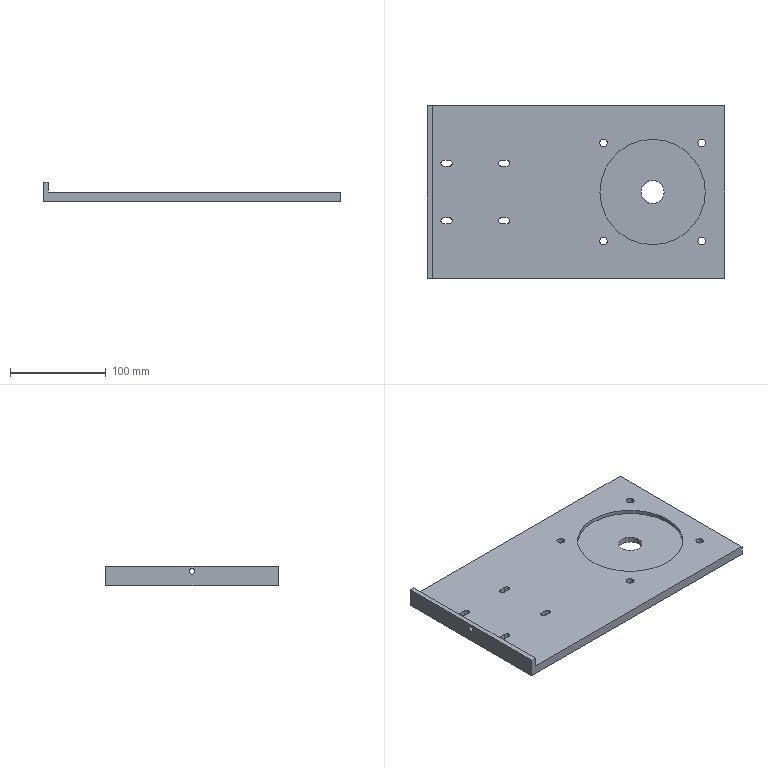Part | STEP file | Motor mounting plate | 1 solid | 43 faces | box 310 x 180 x 20 mm | volume 521549 mm3 | cylinder 26 | plane 17 | commonest cylinder face diameters 6 x14 8 x8 24 x2 110 x2
STEP:
#1=CARTESIAN_POINT('',(-36.,-56.875,10.));
#2=VERTEX_POINT('',#1);
#3=CARTESIAN_POINT('',(-33.,-53.875,10.));
#4=VERTEX_POINT('',#3);
#5=CARTESIAN_POINT('',(-33.,-56.875,10.));
#6=DIRECTION('',(0.,0.,-1.));
#7=DIRECTION('',(-1.,0.,0.));
#8=AXIS2_PLACEMENT_3D('',#5,#6,#7);
#9=CIRCLE('',#8,3.);
#10=EDGE_CURVE('',#2,#4,#9,.T.);
#11=ORIENTED_EDGE('',*,*,#10,.F.);
#12=CARTESIAN_POINT('',(-36.,-56.875,0.));
#13=VERTEX_POINT('',#12);
#14=CARTESIAN_POINT('',(-36.,-56.875,10.));
#15=DIRECTION('',(0.,0.,-1.));
#16=VECTOR('',#15,1000.);
#17=LINE('',#14,#16);
#18=EDGE_CURVE('',#2,#13,#17,.T.);
#19=ORIENTED_EDGE('',*,*,#18,.T.);
#20=CARTESIAN_POINT('',(-33.,-53.875,0.));
#21=VERTEX_POINT('',#20);
#22=CARTESIAN_POINT('',(-33.,-56.875,0.));
#23=DIRECTION('',(0.,0.,-1.));
#24=DIRECTION('',(-1.,0.,0.));
#25=AXIS2_PLACEMENT_3D('',#22,#23,#24);
#26=CIRCLE('',#25,3.);
#27=EDGE_CURVE('',#13,#21,#26,.T.);
#28=ORIENTED_EDGE('',*,*,#27,.T.);
#29=CARTESIAN_POINT('',(-33.,-53.875,10.));
#30=DIRECTION('',(0.,0.,-1.));
#31=VECTOR('',#30,1000.);
#32=LINE('',#29,#31);
#33=EDGE_CURVE('',#4,#21,#32,.T.);
#34=ORIENTED_EDGE('',*,*,#33,.F.);
#35=EDGE_LOOP('',(#11,#19,#28,#34));
#36=FACE_OUTER_BOUND('',#35,.T.);
#37=CARTESIAN_POINT('',(-33.,-56.875,10.));
#38=DIRECTION('',(0.,0.,-1.));
#39=DIRECTION('',(-1.,0.,0.));
#40=AXIS2_PLACEMENT_3D('',#37,#38,#39);
#41=CYLINDRICAL_SURFACE('',#40,3.);
#42=ADVANCED_FACE('',(#36),#41,.F.);
#43=CARTESIAN_POINT('',(-36.,3.125,10.));
#44=VERTEX_POINT('',#43);
#45=CARTESIAN_POINT('',(-33.,6.125,10.));
#46=VERTEX_POINT('',#45);
#47=CARTESIAN_POINT('',(-33.,3.125,10.));
#48=DIRECTION('',(0.,0.,-1.));
#49=DIRECTION('',(-1.,0.,0.));
#50=AXIS2_PLACEMENT_3D('',#47,#48,#49);
#51=CIRCLE('',#50,3.);
#52=EDGE_CURVE('',#44,#46,#51,.T.);
#53=ORIENTED_EDGE('',*,*,#52,.F.);
#54=CARTESIAN_POINT('',(-36.,3.125,0.));
#55=VERTEX_POINT('',#54);
#56=CARTESIAN_POINT('',(-36.,3.125,10.));
#57=DIRECTION('',(0.,0.,-1.));
#58=VECTOR('',#57,1000.);
#59=LINE('',#56,#58);
#60=EDGE_CURVE('',#44,#55,#59,.T.);
#61=ORIENTED_EDGE('',*,*,#60,.T.);
#62=CARTESIAN_POINT('',(-33.,6.125,0.));
#63=VERTEX_POINT('',#62);
#64=CARTESIAN_POINT('',(-33.,3.125,0.));
#65=DIRECTION('',(0.,0.,-1.));
#66=DIRECTION('',(-1.,0.,0.));
#67=AXIS2_PLACEMENT_3D('',#64,#65,#66);
#68=CIRCLE('',#67,3.);
#69=EDGE_CURVE('',#55,#63,#68,.T.);
#70=ORIENTED_EDGE('',*,*,#69,.T.);
#71=CARTESIAN_POINT('',(-33.,6.125,10.));
#72=DIRECTION('',(0.,0.,-1.));
#73=VECTOR('',#72,1000.);
#74=LINE('',#71,#73);
#75=EDGE_CURVE('',#46,#63,#74,.T.);
#76=ORIENTED_EDGE('',*,*,#75,.F.);
#77=EDGE_LOOP('',(#53,#61,#70,#76));
#78=FACE_OUTER_BOUND('',#77,.T.);
#79=CARTESIAN_POINT('',(-33.,3.125,10.));
#80=DIRECTION('',(0.,0.,-1.));
#81=DIRECTION('',(-1.,0.,0.));
#82=AXIS2_PLACEMENT_3D('',#79,#80,#81);
#83=CYLINDRICAL_SURFACE('',#82,3.);
#84=ADVANCED_FACE('',(#78),#83,.F.);
#85=CARTESIAN_POINT('',(240.265,-78.14,10.));
#86=VERTEX_POINT('',#85);
#87=CARTESIAN_POINT('',(232.265,-78.14,10.));
#88=VERTEX_POINT('',#87);
#89=CARTESIAN_POINT('',(236.265,-78.14,10.));
#90=DIRECTION('',(0.,0.,-1.));
#91=DIRECTION('',(-1.,0.,0.));
#92=AXIS2_PLACEMENT_3D('',#89,#90,#91);
#93=CIRCLE('',#92,4.);
#94=EDGE_CURVE('',#86,#88,#93,.T.);
#95=ORIENTED_EDGE('',*,*,#94,.F.);
#96=CARTESIAN_POINT('',(240.265,-78.14,0.));
#97=VERTEX_POINT('',#96);
#98=CARTESIAN_POINT('',(240.265,-78.14,10.));
#99=DIRECTION('',(0.,0.,-1.));
#100=VECTOR('',#99,1000.);
#101=LINE('',#98,#100);
#102=EDGE_CURVE('',#86,#97,#101,.T.);
#103=ORIENTED_EDGE('',*,*,#102,.T.);
#104=CARTESIAN_POINT('',(232.265,-78.14,0.));
#105=VERTEX_POINT('',#104);
#106=CARTESIAN_POINT('',(236.265,-78.14,0.));
#107=DIRECTION('',(0.,0.,-1.));
#108=DIRECTION('',(-1.,0.,0.));
#109=AXIS2_PLACEMENT_3D('',#106,#107,#108);
#110=CIRCLE('',#109,4.);
#111=EDGE_CURVE('',#97,#105,#110,.T.);
#112=ORIENTED_EDGE('',*,*,#111,.T.);
#113=CARTESIAN_POINT('',(232.265,-78.14,10.));
#114=DIRECTION('',(0.,0.,-1.));
#115=VECTOR('',#114,1000.);
#116=LINE('',#113,#115);
#117=EDGE_CURVE('',#88,#105,#116,.T.);
#118=ORIENTED_EDGE('',*,*,#117,.F.);
#119=EDGE_LOOP('',(#95,#103,#112,#118));
#120=FACE_OUTER_BOUND('',#119,.T.);
#121=CARTESIAN_POINT('',(236.265,-78.14,10.));
#122=DIRECTION('',(0.,0.,-1.));
#123=DIRECTION('',(-1.,0.,0.));
#124=AXIS2_PLACEMENT_3D('',#121,#122,#123);
#125=CYLINDRICAL_SURFACE('',#124,4.);
#126=ADVANCED_FACE('',(#120),#125,.F.);
#127=CARTESIAN_POINT('',(137.735,24.39,10.));
#128=VERTEX_POINT('',#127);
#129=CARTESIAN_POINT('',(129.735,24.39,10.));
#130=VERTEX_POINT('',#129);
#131=CARTESIAN_POINT('',(133.735,24.39,10.));
#132=DIRECTION('',(0.,0.,-1.));
#133=DIRECTION('',(-1.,0.,0.));
#134=AXIS2_PLACEMENT_3D('',#131,#132,#133);
#135=CIRCLE('',#134,4.);
#136=EDGE_CURVE('',#128,#130,#135,.T.);
#137=ORIENTED_EDGE('',*,*,#136,.F.);
#138=CARTESIAN_POINT('',(137.735,24.39,0.));
#139=VERTEX_POINT('',#138);
#140=CARTESIAN_POINT('',(137.735,24.39,10.));
#141=DIRECTION('',(0.,0.,-1.));
#142=VECTOR('',#141,1000.);
#143=LINE('',#140,#142);
#144=EDGE_CURVE('',#128,#139,#143,.T.);
#145=ORIENTED_EDGE('',*,*,#144,.T.);
#146=CARTESIAN_POINT('',(129.735,24.39,0.));
#147=VERTEX_POINT('',#146);
#148=CARTESIAN_POINT('',(133.735,24.39,0.));
#149=DIRECTION('',(0.,0.,-1.));
#150=DIRECTION('',(-1.,0.,0.));
#151=AXIS2_PLACEMENT_3D('',#148,#149,#150);
#152=CIRCLE('',#151,4.);
#153=EDGE_CURVE('',#139,#147,#152,.T.);
#154=ORIENTED_EDGE('',*,*,#153,.T.);
#155=CARTESIAN_POINT('',(129.735,24.39,10.));
#156=DIRECTION('',(0.,0.,-1.));
#157=VECTOR('',#156,1000.);
#158=LINE('',#155,#157);
#159=EDGE_CURVE('',#130,#147,#158,.T.);
#160=ORIENTED_EDGE('',*,*,#159,.F.);
#161=EDGE_LOOP('',(#137,#145,#154,#160));
#162=FACE_OUTER_BOUND('',#161,.T.);
#163=CARTESIAN_POINT('',(133.735,24.39,10.));
#164=DIRECTION('',(0.,0.,-1.));
#165=DIRECTION('',(-1.,0.,0.));
#166=AXIS2_PLACEMENT_3D('',#163,#164,#165);
#167=CYLINDRICAL_SURFACE('',#166,4.);
#168=ADVANCED_FACE('',(#162),#167,.F.);
#169=CARTESIAN_POINT('',(197.,-26.875,6.));
#170=VERTEX_POINT('',#169);
#171=CARTESIAN_POINT('',(173.,-26.875,6.));
#172=VERTEX_POINT('',#171);
#173=CARTESIAN_POINT('',(185.,-26.875,6.));
#174=DIRECTION('',(0.,0.,-1.));
#175=DIRECTION('',(-1.,0.,0.));
#176=AXIS2_PLACEMENT_3D('',#173,#174,#175);
#177=CIRCLE('',#176,12.);
#178=EDGE_CURVE('',#170,#172,#177,.T.);
#179=ORIENTED_EDGE('',*,*,#178,.F.);
#180=CARTESIAN_POINT('',(197.,-26.875,0.));
#181=VERTEX_POINT('',#180);
#182=CARTESIAN_POINT('',(197.,-26.875,10.));
#183=DIRECTION('',(0.,0.,-1.));
#184=VECTOR('',#183,1000.);
#185=LINE('',#182,#184);
#186=EDGE_CURVE('',#170,#181,#185,.T.);
#187=ORIENTED_EDGE('',*,*,#186,.T.);
#188=CARTESIAN_POINT('',(173.,-26.875,0.));
#189=VERTEX_POINT('',#188);
#190=CARTESIAN_POINT('',(185.,-26.875,0.));
#191=DIRECTION('',(0.,0.,-1.));
#192=DIRECTION('',(-1.,0.,0.));
#193=AXIS2_PLACEMENT_3D('',#190,#191,#192);
#194=CIRCLE('',#193,12.);
#195=EDGE_CURVE('',#181,#189,#194,.T.);
#196=ORIENTED_EDGE('',*,*,#195,.T.);
#197=CARTESIAN_POINT('',(173.,-26.875,10.));
#198=DIRECTION('',(0.,0.,-1.));
#199=VECTOR('',#198,1000.);
#200=LINE('',#197,#199);
#201=EDGE_CURVE('',#172,#189,#200,.T.);
#202=ORIENTED_EDGE('',*,*,#201,.F.);
#203=EDGE_LOOP('',(#179,#187,#196,#202));
#204=FACE_OUTER_BOUND('',#203,.T.);
#205=CARTESIAN_POINT('',(185.,-26.875,10.));
#206=DIRECTION('',(0.,0.,-1.));
#207=DIRECTION('',(-1.,0.,0.));
#208=AXIS2_PLACEMENT_3D('',#205,#206,#207);
#209=CYLINDRICAL_SURFACE('',#208,12.);
#210=ADVANCED_FACE('',(#204),#209,.F.);
#211=CARTESIAN_POINT('',(24.,3.125,10.));
#212=VERTEX_POINT('',#211);
#213=CARTESIAN_POINT('',(27.,6.125,10.));
#214=VERTEX_POINT('',#213);
#215=CARTESIAN_POINT('',(27.,3.125,10.));
#216=DIRECTION('',(0.,0.,-1.));
#217=DIRECTION('',(-1.,0.,0.));
#218=AXIS2_PLACEMENT_3D('',#215,#216,#217);
#219=CIRCLE('',#218,3.);
#220=EDGE_CURVE('',#212,#214,#219,.T.);
#221=ORIENTED_EDGE('',*,*,#220,.F.);
#222=CARTESIAN_POINT('',(24.,3.125,0.));
#223=VERTEX_POINT('',#222);
#224=CARTESIAN_POINT('',(24.,3.125,10.));
#225=DIRECTION('',(0.,0.,-1.));
#226=VECTOR('',#225,1000.);
#227=LINE('',#224,#226);
#228=EDGE_CURVE('',#212,#223,#227,.T.);
#229=ORIENTED_EDGE('',*,*,#228,.T.);
#230=CARTESIAN_POINT('',(27.,6.125,0.));
#231=VERTEX_POINT('',#230);
#232=CARTESIAN_POINT('',(27.,3.125,0.));
#233=DIRECTION('',(0.,0.,-1.));
#234=DIRECTION('',(-1.,0.,0.));
#235=AXIS2_PLACEMENT_3D('',#232,#233,#234);
#236=CIRCLE('',#235,3.);
#237=EDGE_CURVE('',#223,#231,#236,.T.);
#238=ORIENTED_EDGE('',*,*,#237,.T.);
#239=CARTESIAN_POINT('',(27.,6.125,10.));
#240=DIRECTION('',(0.,0.,-1.));
#241=VECTOR('',#240,1000.);
#242=LINE('',#239,#241);
#243=EDGE_CURVE('',#214,#231,#242,.T.);
#244=ORIENTED_EDGE('',*,*,#243,.F.);
#245=EDGE_LOOP('',(#221,#229,#238,#244));
#246=FACE_OUTER_BOUND('',#245,.T.);
#247=CARTESIAN_POINT('',(27.,3.125,10.));
#248=DIRECTION('',(0.,0.,-1.));
#249=DIRECTION('',(-1.,0.,0.));
#250=AXIS2_PLACEMENT_3D('',#247,#248,#249);
#251=CYLINDRICAL_SURFACE('',#250,3.);
#252=ADVANCED_FACE('',(#246),#251,.F.);
#253=CARTESIAN_POINT('',(240.265,24.39,10.));
#254=VERTEX_POINT('',#253);
#255=CARTESIAN_POINT('',(232.265,24.39,10.));
#256=VERTEX_POINT('',#255);
#257=CARTESIAN_POINT('',(236.265,24.39,10.));
#258=DIRECTION('',(0.,0.,-1.));
#259=DIRECTION('',(-1.,0.,0.));
#260=AXIS2_PLACEMENT_3D('',#257,#258,#259);
#261=CIRCLE('',#260,4.);
#262=EDGE_CURVE('',#254,#256,#261,.T.);
#263=ORIENTED_EDGE('',*,*,#262,.F.);
#264=CARTESIAN_POINT('',(240.265,24.39,0.));
#265=VERTEX_POINT('',#264);
#266=CARTESIAN_POINT('',(240.265,24.39,10.));
#267=DIRECTION('',(0.,0.,-1.));
#268=VECTOR('',#267,1000.);
#269=LINE('',#266,#268);
#270=EDGE_CURVE('',#254,#265,#269,.T.);
#271=ORIENTED_EDGE('',*,*,#270,.T.);
#272=CARTESIAN_POINT('',(232.265,24.39,0.));
#273=VERTEX_POINT('',#272);
#274=CARTESIAN_POINT('',(236.265,24.39,0.));
#275=DIRECTION('',(0.,0.,-1.));
#276=DIRECTION('',(-1.,0.,0.));
#277=AXIS2_PLACEMENT_3D('',#274,#275,#276);
#278=CIRCLE('',#277,4.);
#279=EDGE_CURVE('',#265,#273,#278,.T.);
#280=ORIENTED_EDGE('',*,*,#279,.T.);
#281=CARTESIAN_POINT('',(232.265,24.39,10.));
#282=DIRECTION('',(0.,0.,-1.));
#283=VECTOR('',#282,1000.);
#284=LINE('',#281,#283);
#285=EDGE_CURVE('',#256,#273,#284,.T.);
#286=ORIENTED_EDGE('',*,*,#285,.F.);
#287=EDGE_LOOP('',(#263,#271,#280,#286));
#288=FACE_OUTER_BOUND('',#287,.T.);
#289=CARTESIAN_POINT('',(236.265,24.39,10.));
#290=DIRECTION('',(0.,0.,-1.));
#291=DIRECTION('',(-1.,0.,0.));
#292=AXIS2_PLACEMENT_3D('',#289,#290,#291);
#293=CYLINDRICAL_SURFACE('',#292,4.);
#294=ADVANCED_FACE('',(#288),#293,.F.);
#295=CARTESIAN_POINT('',(137.735,-78.14,10.));
#296=VERTEX_POINT('',#295);
#297=CARTESIAN_POINT('',(129.735,-78.14,10.));
#298=VERTEX_POINT('',#297);
#299=CARTESIAN_POINT('',(133.735,-78.14,10.));
#300=DIRECTION('',(0.,0.,-1.));
#301=DIRECTION('',(-1.,0.,0.));
#302=AXIS2_PLACEMENT_3D('',#299,#300,#301);
#303=CIRCLE('',#302,4.);
#304=EDGE_CURVE('',#296,#298,#303,.T.);
#305=ORIENTED_EDGE('',*,*,#304,.F.);
#306=CARTESIAN_POINT('',(137.735,-78.14,0.));
#307=VERTEX_POINT('',#306);
#308=CARTESIAN_POINT('',(137.735,-78.14,10.));
#309=DIRECTION('',(0.,0.,-1.));
#310=VECTOR('',#309,1000.);
#311=LINE('',#308,#310);
#312=EDGE_CURVE('',#296,#307,#311,.T.);
#313=ORIENTED_EDGE('',*,*,#312,.T.);
#314=CARTESIAN_POINT('',(129.735,-78.14,0.));
#315=VERTEX_POINT('',#314);
#316=CARTESIAN_POINT('',(133.735,-78.14,0.));
#317=DIRECTION('',(0.,0.,-1.));
#318=DIRECTION('',(-1.,0.,0.));
#319=AXIS2_PLACEMENT_3D('',#316,#317,#318);
#320=CIRCLE('',#319,4.);
#321=EDGE_CURVE('',#307,#315,#320,.T.);
#322=ORIENTED_EDGE('',*,*,#321,.T.);
#323=CARTESIAN_POINT('',(129.735,-78.14,10.));
#324=DIRECTION('',(0.,0.,-1.));
#325=VECTOR('',#324,1000.);
#326=LINE('',#323,#325);
#327=EDGE_CURVE('',#298,#315,#326,.T.);
#328=ORIENTED_EDGE('',*,*,#327,.F.);
#329=EDGE_LOOP('',(#305,#313,#322,#328));
#330=FACE_OUTER_BOUND('',#329,.T.);
#331=CARTESIAN_POINT('',(133.735,-78.14,10.));
#332=DIRECTION('',(0.,0.,-1.));
#333=DIRECTION('',(-1.,0.,0.));
#334=AXIS2_PLACEMENT_3D('',#331,#332,#333);
#335=CYLINDRICAL_SURFACE('',#334,4.);
#336=ADVANCED_FACE('',(#330),#335,.F.);
#337=CARTESIAN_POINT('',(24.,-56.875,10.));
#338=VERTEX_POINT('',#337);
#339=CARTESIAN_POINT('',(27.,-53.875,10.));
#340=VERTEX_POINT('',#339);
#341=CARTESIAN_POINT('',(27.,-56.875,10.));
#342=DIRECTION('',(0.,0.,-1.));
#343=DIRECTION('',(-1.,0.,0.));
#344=AXIS2_PLACEMENT_3D('',#341,#342,#343);
#345=CIRCLE('',#344,3.);
#346=EDGE_CURVE('',#338,#340,#345,.T.);
#347=ORIENTED_EDGE('',*,*,#346,.F.);
#348=CARTESIAN_POINT('',(24.,-56.875,0.));
#349=VERTEX_POINT('',#348);
#350=CARTESIAN_POINT('',(24.,-56.875,10.));
#351=DIRECTION('',(0.,0.,-1.));
#352=VECTOR('',#351,1000.);
#353=LINE('',#350,#352);
#354=EDGE_CURVE('',#338,#349,#353,.T.);
#355=ORIENTED_EDGE('',*,*,#354,.T.);
#356=CARTESIAN_POINT('',(27.,-53.875,0.));
#357=VERTEX_POINT('',#356);
#358=CARTESIAN_POINT('',(27.,-56.875,0.));
#359=DIRECTION('',(0.,0.,-1.));
#360=DIRECTION('',(-1.,0.,0.));
#361=AXIS2_PLACEMENT_3D('',#358,#359,#360);
#362=CIRCLE('',#361,3.);
#363=EDGE_CURVE('',#349,#357,#362,.T.);
#364=ORIENTED_EDGE('',*,*,#363,.T.);
#365=CARTESIAN_POINT('',(27.,-53.875,10.));
#366=DIRECTION('',(0.,0.,-1.));
#367=VECTOR('',#366,1000.);
#368=LINE('',#365,#367);
#369=EDGE_CURVE('',#340,#357,#368,.T.);
#370=ORIENTED_EDGE('',*,*,#369,.F.);
#371=EDGE_LOOP('',(#347,#355,#364,#370));
#372=FACE_OUTER_BOUND('',#371,.T.);
#373=CARTESIAN_POINT('',(27.,-56.875,10.));
#374=DIRECTION('',(0.,0.,-1.));
#375=DIRECTION('',(-1.,0.,0.));
#376=AXIS2_PLACEMENT_3D('',#373,#374,#375);
#377=CYLINDRICAL_SURFACE('',#376,3.);
#378=ADVANCED_FACE('',(#372),#377,.F.);
#379=CARTESIAN_POINT('',(-45.,-26.875,12.));
#380=VERTEX_POINT('',#379);
#381=CARTESIAN_POINT('',(-45.,-26.875,18.));
#382=VERTEX_POINT('',#381);
#383=CARTESIAN_POINT('',(-45.,-26.875,15.));
#384=DIRECTION('',(-1.,0.,0.));
#385=DIRECTION('',(0.,0.,1.));
#386=AXIS2_PLACEMENT_3D('',#383,#384,#385);
#387=CIRCLE('',#386,3.);
#388=EDGE_CURVE('',#380,#382,#387,.T.);
#389=ORIENTED_EDGE('',*,*,#388,.F.);
#390=CARTESIAN_POINT('',(-50.,-26.875,12.));
#391=VERTEX_POINT('',#390);
#392=CARTESIAN_POINT('',(-45.,-26.875,12.));
#393=DIRECTION('',(-1.,0.,0.));
#394=VECTOR('',#393,1000.);
#395=LINE('',#392,#394);
#396=EDGE_CURVE('',#380,#391,#395,.T.);
#397=ORIENTED_EDGE('',*,*,#396,.T.);
#398=CARTESIAN_POINT('',(-50.,-26.875,18.));
#399=VERTEX_POINT('',#398);
#400=CARTESIAN_POINT('',(-50.,-26.875,15.));
#401=DIRECTION('',(-1.,0.,0.));
#402=DIRECTION('',(0.,0.,1.));
#403=AXIS2_PLACEMENT_3D('',#400,#401,#402);
#404=CIRCLE('',#403,3.);
#405=EDGE_CURVE('',#391,#399,#404,.T.);
#406=ORIENTED_EDGE('',*,*,#405,.T.);
#407=CARTESIAN_POINT('',(-45.,-26.875,18.));
#408=DIRECTION('',(-1.,0.,0.));
#409=VECTOR('',#408,1000.);
#410=LINE('',#407,#409);
#411=EDGE_CURVE('',#382,#399,#410,.T.);
#412=ORIENTED_EDGE('',*,*,#411,.F.);
#413=EDGE_LOOP('',(#389,#397,#406,#412));
#414=FACE_OUTER_BOUND('',#413,.T.);
#415=CARTESIAN_POINT('',(-45.,-26.875,15.));
#416=DIRECTION('',(-1.,0.,0.));
#417=DIRECTION('',(0.,0.,1.));
#418=AXIS2_PLACEMENT_3D('',#415,#416,#417);
#419=CYLINDRICAL_SURFACE('',#418,3.);
#420=ADVANCED_FACE('',(#414),#419,.F.);
#421=CARTESIAN_POINT('',(130.,-26.875,6.));
#422=VERTEX_POINT('',#421);
#423=CARTESIAN_POINT('',(240.,-26.875,6.));
#424=VERTEX_POINT('',#423);
#425=CARTESIAN_POINT('',(185.,-26.875,6.));
#426=DIRECTION('',(0.,0.,1.));
#427=DIRECTION('',(1.,0.,0.));
#428=AXIS2_PLACEMENT_3D('',#425,#426,#427);
#429=CIRCLE('',#428,55.);
#430=EDGE_CURVE('',#422,#424,#429,.T.);
#431=ORIENTED_EDGE('',*,*,#430,.F.);
#432=CARTESIAN_POINT('',(130.,-26.875,10.));
#433=VERTEX_POINT('',#432);
#434=CARTESIAN_POINT('',(130.,-26.875,6.));
#435=DIRECTION('',(0.,0.,1.));
#436=VECTOR('',#435,1000.);
#437=LINE('',#434,#436);
#438=EDGE_CURVE('',#422,#433,#437,.T.);
#439=ORIENTED_EDGE('',*,*,#438,.T.);
#440=CARTESIAN_POINT('',(240.,-26.875,10.));
#441=VERTEX_POINT('',#440);
#442=CARTESIAN_POINT('',(185.,-26.875,10.));
#443=DIRECTION('',(0.,0.,-1.));
#444=DIRECTION('',(1.,0.,0.));
#445=AXIS2_PLACEMENT_3D('',#442,#443,#444);
#446=CIRCLE('',#445,55.);
#447=EDGE_CURVE('',#441,#433,#446,.T.);
#448=ORIENTED_EDGE('',*,*,#447,.F.);
#449=CARTESIAN_POINT('',(240.,-26.875,6.));
#450=DIRECTION('',(0.,0.,1.));
#451=VECTOR('',#450,1000.);
#452=LINE('',#449,#451);
#453=EDGE_CURVE('',#424,#441,#452,.T.);
#454=ORIENTED_EDGE('',*,*,#453,.F.);
#455=EDGE_LOOP('',(#431,#439,#448,#454));
#456=FACE_OUTER_BOUND('',#455,.T.);
#457=CARTESIAN_POINT('',(185.,-26.875,6.));
#458=DIRECTION('',(0.,0.,1.));
#459=DIRECTION('',(1.,0.,0.));
#460=AXIS2_PLACEMENT_3D('',#457,#458,#459);
#461=CYLINDRICAL_SURFACE('',#460,55.);
#462=ADVANCED_FACE('',(#456),#461,.F.);
#463=CARTESIAN_POINT('',(-27.,-53.875,0.));
#464=VERTEX_POINT('',#463);
#465=CARTESIAN_POINT('',(-50.,-53.875,0.));
#466=DIRECTION('',(1.,0.,0.));
#467=VECTOR('',#466,1000.);
#468=LINE('',#465,#467);
#469=EDGE_CURVE('',#21,#464,#468,.T.);
#470=ORIENTED_EDGE('',*,*,#469,.F.);
#471=ORIENTED_EDGE('',*,*,#27,.F.);
#472=CARTESIAN_POINT('',(-33.,-59.875,0.));
#473=VERTEX_POINT('',#472);
#474=CARTESIAN_POINT('',(-33.,-56.875,0.));
#475=DIRECTION('',(0.,0.,-1.));
#476=DIRECTION('',(-1.,0.,0.));
#477=AXIS2_PLACEMENT_3D('',#474,#475,#476);
#478=CIRCLE('',#477,3.);
#479=EDGE_CURVE('',#473,#13,#478,.T.);
#480=ORIENTED_EDGE('',*,*,#479,.F.);
#481=CARTESIAN_POINT('',(-27.,-59.875,0.));
#482=VERTEX_POINT('',#481);
#483=CARTESIAN_POINT('',(-50.,-59.875,0.));
#484=DIRECTION('',(-1.,0.,0.));
#485=VECTOR('',#484,1000.);
#486=LINE('',#483,#485);
#487=EDGE_CURVE('',#482,#473,#486,.T.);
#488=ORIENTED_EDGE('',*,*,#487,.F.);
#489=CARTESIAN_POINT('',(-27.,-56.875,0.));
#490=DIRECTION('',(0.,0.,-1.));
#491=DIRECTION('',(-1.,0.,0.));
#492=AXIS2_PLACEMENT_3D('',#489,#490,#491);
#493=CIRCLE('',#492,3.);
#494=EDGE_CURVE('',#464,#482,#493,.T.);
#495=ORIENTED_EDGE('',*,*,#494,.F.);
#496=EDGE_LOOP('',(#470,#471,#480,#488,#495));
#497=FACE_BOUND('',#496,.T.);
#498=CARTESIAN_POINT('',(-27.,6.125,0.));
#499=VERTEX_POINT('',#498);
#500=CARTESIAN_POINT('',(-50.,6.125,0.));
#501=DIRECTION('',(1.,0.,0.));
#502=VECTOR('',#501,1000.);
#503=LINE('',#500,#502);
#504=EDGE_CURVE('',#63,#499,#503,.T.);
#505=ORIENTED_EDGE('',*,*,#504,.F.);
#506=ORIENTED_EDGE('',*,*,#69,.F.);
#507=CARTESIAN_POINT('',(-33.,0.1251,0.));
#508=VERTEX_POINT('',#507);
#509=CARTESIAN_POINT('',(-33.,3.125,0.));
#510=DIRECTION('',(0.,0.,-1.));
#511=DIRECTION('',(-1.,0.,0.));
#512=AXIS2_PLACEMENT_3D('',#509,#510,#511);
#513=CIRCLE('',#512,3.);
#514=EDGE_CURVE('',#508,#55,#513,.T.);
#515=ORIENTED_EDGE('',*,*,#514,.F.);
#516=CARTESIAN_POINT('',(-27.,0.1251,0.));
#517=VERTEX_POINT('',#516);
#518=CARTESIAN_POINT('',(-50.,0.1251,0.));
#519=DIRECTION('',(-1.,0.,0.));
#520=VECTOR('',#519,1000.);
#521=LINE('',#518,#520);
#522=EDGE_CURVE('',#517,#508,#521,.T.);
#523=ORIENTED_EDGE('',*,*,#522,.F.);
#524=CARTESIAN_POINT('',(-27.,3.125,0.));
#525=DIRECTION('',(0.,0.,-1.));
#526=DIRECTION('',(-1.,0.,0.));
#527=AXIS2_PLACEMENT_3D('',#524,#525,#526);
#528=CIRCLE('',#527,3.);
#529=EDGE_CURVE('',#499,#517,#528,.T.);
#530=ORIENTED_EDGE('',*,*,#529,.F.);
#531=EDGE_LOOP('',(#505,#506,#515,#523,#530));
#532=FACE_BOUND('',#531,.T.);
#533=CARTESIAN_POINT('',(236.265,-78.14,0.));
#534=DIRECTION('',(0.,0.,-1.));
#535=DIRECTION('',(-1.,0.,0.));
#536=AXIS2_PLACEMENT_3D('',#533,#534,#535);
#537=CIRCLE('',#536,4.);
#538=EDGE_CURVE('',#105,#97,#537,.T.);
#539=ORIENTED_EDGE('',*,*,#538,.F.);
#540=ORIENTED_EDGE('',*,*,#111,.F.);
#541=EDGE_LOOP('',(#539,#540));
#542=FACE_BOUND('',#541,.T.);
#543=CARTESIAN_POINT('',(133.735,24.39,0.));
#544=DIRECTION('',(0.,0.,-1.));
#545=DIRECTION('',(-1.,0.,0.));
#546=AXIS2_PLACEMENT_3D('',#543,#544,#545);
#547=CIRCLE('',#546,4.);
#548=EDGE_CURVE('',#147,#139,#547,.T.);
#549=ORIENTED_EDGE('',*,*,#548,.F.);
#550=ORIENTED_EDGE('',*,*,#153,.F.);
#551=EDGE_LOOP('',(#549,#550));
#552=FACE_BOUND('',#551,.T.);
#553=CARTESIAN_POINT('',(185.,-26.875,0.));
#554=DIRECTION('',(0.,0.,-1.));
#555=DIRECTION('',(-1.,0.,0.));
#556=AXIS2_PLACEMENT_3D('',#553,#554,#555);
#557=CIRCLE('',#556,12.);
#558=EDGE_CURVE('',#189,#181,#557,.T.);
#559=ORIENTED_EDGE('',*,*,#558,.F.);
#560=ORIENTED_EDGE('',*,*,#195,.F.);
#561=EDGE_LOOP('',(#559,#560));
#562=FACE_BOUND('',#561,.T.);
#563=CARTESIAN_POINT('',(260.,63.125,0.));
#564=VERTEX_POINT('',#563);
#565=CARTESIAN_POINT('',(-50.,63.125,0.));
#566=VERTEX_POINT('',#565);
#567=CARTESIAN_POINT('',(-50.,63.125,0.));
#568=DIRECTION('',(-1.,0.,0.));
#569=VECTOR('',#568,1000.);
#570=LINE('',#567,#569);
#571=EDGE_CURVE('',#564,#566,#570,.T.);
#572=ORIENTED_EDGE('',*,*,#571,.F.);
#573=CARTESIAN_POINT('',(260.,-116.875,0.));
#574=VERTEX_POINT('',#573);
#575=CARTESIAN_POINT('',(260.,-116.875,0.));
#576=DIRECTION('',(0.,1.,0.));
#577=VECTOR('',#576,1000.);
#578=LINE('',#575,#577);
#579=EDGE_CURVE('',#574,#564,#578,.T.);
#580=ORIENTED_EDGE('',*,*,#579,.F.);
#581=CARTESIAN_POINT('',(-50.,-116.875,0.));
#582=VERTEX_POINT('',#581);
#583=CARTESIAN_POINT('',(-50.,-116.875,0.));
#584=DIRECTION('',(1.,0.,0.));
#585=VECTOR('',#584,1000.);
#586=LINE('',#583,#585);
#587=EDGE_CURVE('',#582,#574,#586,.T.);
#588=ORIENTED_EDGE('',*,*,#587,.F.);
#589=CARTESIAN_POINT('',(-50.,-116.875,0.));
#590=DIRECTION('',(0.,-1.,0.));
#591=VECTOR('',#590,1000.);
#592=LINE('',#589,#591);
#593=EDGE_CURVE('',#566,#582,#592,.T.);
#594=ORIENTED_EDGE('',*,*,#593,.F.);
#595=EDGE_LOOP('',(#572,#580,#588,#594));
#596=FACE_OUTER_BOUND('',#595,.T.);
#597=CARTESIAN_POINT('',(33.,6.125,0.));
#598=VERTEX_POINT('',#597);
#599=CARTESIAN_POINT('',(-50.,6.125,0.));
#600=DIRECTION('',(1.,0.,0.));
#601=VECTOR('',#600,1000.);
#602=LINE('',#599,#601);
#603=EDGE_CURVE('',#231,#598,#602,.T.);
#604=ORIENTED_EDGE('',*,*,#603,.F.);
#605=ORIENTED_EDGE('',*,*,#237,.F.);
#606=CARTESIAN_POINT('',(27.,0.1251,0.));
#607=VERTEX_POINT('',#606);
#608=CARTESIAN_POINT('',(27.,3.125,0.));
#609=DIRECTION('',(0.,0.,-1.));
#610=DIRECTION('',(-1.,0.,0.));
#611=AXIS2_PLACEMENT_3D('',#608,#609,#610);
#612=CIRCLE('',#611,3.);
#613=EDGE_CURVE('',#607,#223,#612,.T.);
#614=ORIENTED_EDGE('',*,*,#613,.F.);
#615=CARTESIAN_POINT('',(33.,0.1251,0.));
#616=VERTEX_POINT('',#615);
#617=CARTESIAN_POINT('',(-50.,0.1251,0.));
#618=DIRECTION('',(-1.,0.,0.));
#619=VECTOR('',#618,1000.);
#620=LINE('',#617,#619);
#621=EDGE_CURVE('',#616,#607,#620,.T.);
#622=ORIENTED_EDGE('',*,*,#621,.F.);
#623=CARTESIAN_POINT('',(33.,3.125,0.));
#624=DIRECTION('',(0.,0.,-1.));
#625=DIRECTION('',(-1.,0.,0.));
#626=AXIS2_PLACEMENT_3D('',#623,#624,#625);
#627=CIRCLE('',#626,3.);
#628=EDGE_CURVE('',#598,#616,#627,.T.);
#629=ORIENTED_EDGE('',*,*,#628,.F.);
#630=EDGE_LOOP('',(#604,#605,#614,#622,#629));
#631=FACE_BOUND('',#630,.T.);
#632=CARTESIAN_POINT('',(236.265,24.39,0.));
#633=DIRECTION('',(0.,0.,-1.));
#634=DIRECTION('',(-1.,0.,0.));
#635=AXIS2_PLACEMENT_3D('',#632,#633,#634);
#636=CIRCLE('',#635,4.);
#637=EDGE_CURVE('',#273,#265,#636,.T.);
#638=ORIENTED_EDGE('',*,*,#637,.F.);
#639=ORIENTED_EDGE('',*,*,#279,.F.);
#640=EDGE_LOOP('',(#638,#639));
#641=FACE_BOUND('',#640,.T.);
#642=CARTESIAN_POINT('',(133.735,-78.14,0.));
#643=DIRECTION('',(0.,0.,-1.));
#644=DIRECTION('',(-1.,0.,0.));
#645=AXIS2_PLACEMENT_3D('',#642,#643,#644);
#646=CIRCLE('',#645,4.);
#647=EDGE_CURVE('',#315,#307,#646,.T.);
#648=ORIENTED_EDGE('',*,*,#647,.F.);
#649=ORIENTED_EDGE('',*,*,#321,.F.);
#650=EDGE_LOOP('',(#648,#649));
#651=FACE_BOUND('',#650,.T.);
#652=CARTESIAN_POINT('',(33.,-53.875,0.));
#653=VERTEX_POINT('',#652);
#654=CARTESIAN_POINT('',(-50.,-53.875,0.));
#655=DIRECTION('',(1.,0.,0.));
#656=VECTOR('',#655,1000.);
#657=LINE('',#654,#656);
#658=EDGE_CURVE('',#357,#653,#657,.T.);
#659=ORIENTED_EDGE('',*,*,#658,.F.);
#660=ORIENTED_EDGE('',*,*,#363,.F.);
#661=CARTESIAN_POINT('',(27.,-59.875,0.));
#662=VERTEX_POINT('',#661);
#663=CARTESIAN_POINT('',(27.,-56.875,0.));
#664=DIRECTION('',(0.,0.,-1.));
#665=DIRECTION('',(-1.,0.,0.));
#666=AXIS2_PLACEMENT_3D('',#663,#664,#665);
#667=CIRCLE('',#666,3.);
#668=EDGE_CURVE('',#662,#349,#667,.T.);
#669=ORIENTED_EDGE('',*,*,#668,.F.);
#670=CARTESIAN_POINT('',(33.,-59.875,0.));
#671=VERTEX_POINT('',#670);
#672=CARTESIAN_POINT('',(-50.,-59.875,0.));
#673=DIRECTION('',(-1.,0.,0.));
#674=VECTOR('',#673,1000.);
#675=LINE('',#672,#674);
#676=EDGE_CURVE('',#671,#662,#675,.T.);
#677=ORIENTED_EDGE('',*,*,#676,.F.);
#678=CARTESIAN_POINT('',(33.,-56.875,0.));
#679=DIRECTION('',(0.,0.,-1.));
#680=DIRECTION('',(-1.,0.,0.));
#681=AXIS2_PLACEMENT_3D('',#678,#679,#680);
#682=CIRCLE('',#681,3.);
#683=EDGE_CURVE('',#653,#671,#682,.T.);
#684=ORIENTED_EDGE('',*,*,#683,.F.);
#685=EDGE_LOOP('',(#659,#660,#669,#677,#684));
#686=FACE_BOUND('',#685,.T.);
#687=CARTESIAN_POINT('',(-50.,-116.875,0.));
#688=DIRECTION('',(0.,0.,1.));
#689=DIRECTION('',(1.,0.,0.));
#690=AXIS2_PLACEMENT_3D('',#687,#688,#689);
#691=PLANE('',#690);
#692=ADVANCED_FACE('',(#497,#532,#542,#552,#562,#596,#631,#641,#651,#686),#691,.F.);
#693=CARTESIAN_POINT('',(-27.,-59.875,10.));
#694=VERTEX_POINT('',#693);
#695=CARTESIAN_POINT('',(-27.,-59.875,10.));
#696=DIRECTION('',(0.,0.,-1.));
#697=VECTOR('',#696,1000.);
#698=LINE('',#695,#697);
#699=EDGE_CURVE('',#694,#482,#698,.T.);
#700=ORIENTED_EDGE('',*,*,#699,.F.);
#701=CARTESIAN_POINT('',(-27.,-53.875,10.));
#702=VERTEX_POINT('',#701);
#703=CARTESIAN_POINT('',(-27.,-56.875,10.));
#704=DIRECTION('',(0.,0.,-1.));
#705=DIRECTION('',(-1.,0.,0.));
#706=AXIS2_PLACEMENT_3D('',#703,#704,#705);
#707=CIRCLE('',#706,3.);
#708=EDGE_CURVE('',#702,#694,#707,.T.);
#709=ORIENTED_EDGE('',*,*,#708,.F.);
#710=CARTESIAN_POINT('',(-27.,-53.875,10.));
#711=DIRECTION('',(0.,0.,1.));
#712=VECTOR('',#711,1000.);
#713=LINE('',#710,#712);
#714=EDGE_CURVE('',#464,#702,#713,.T.);
#715=ORIENTED_EDGE('',*,*,#714,.F.);
#716=ORIENTED_EDGE('',*,*,#494,.T.);
#717=EDGE_LOOP('',(#700,#709,#715,#716));
#718=FACE_OUTER_BOUND('',#717,.T.);
#719=CARTESIAN_POINT('',(-27.,-56.875,10.));
#720=DIRECTION('',(0.,0.,-1.));
#721=DIRECTION('',(-1.,0.,0.));
#722=AXIS2_PLACEMENT_3D('',#719,#720,#721);
#723=CYLINDRICAL_SURFACE('',#722,3.);
#724=ADVANCED_FACE('',(#718),#723,.F.);
#725=CARTESIAN_POINT('',(-27.,-53.875,10.));
#726=DIRECTION('',(-1.,0.,0.));
#727=VECTOR('',#726,1000.);
#728=LINE('',#725,#727);
#729=EDGE_CURVE('',#702,#4,#728,.T.);
#730=ORIENTED_EDGE('',*,*,#729,.T.);
#731=ORIENTED_EDGE('',*,*,#33,.T.);
#732=ORIENTED_EDGE('',*,*,#469,.T.);
#733=ORIENTED_EDGE('',*,*,#714,.T.);
#734=EDGE_LOOP('',(#730,#731,#732,#733));
#735=FACE_OUTER_BOUND('',#734,.T.);
#736=CARTESIAN_POINT('',(-27.,-53.875,10.));
#737=DIRECTION('',(0.,-1.,0.));
#738=DIRECTION('',(0.,0.,-1.));
#739=AXIS2_PLACEMENT_3D('',#736,#737,#738);
#740=PLANE('',#739);
#741=ADVANCED_FACE('',(#735),#740,.T.);
#742=ORIENTED_EDGE('',*,*,#18,.F.);
#743=CARTESIAN_POINT('',(-33.,-59.875,10.));
#744=VERTEX_POINT('',#743);
#745=CARTESIAN_POINT('',(-33.,-56.875,10.));
#746=DIRECTION('',(0.,0.,-1.));
#747=DIRECTION('',(-1.,0.,0.));
#748=AXIS2_PLACEMENT_3D('',#745,#746,#747);
#749=CIRCLE('',#748,3.);
#750=EDGE_CURVE('',#744,#2,#749,.T.);
#751=ORIENTED_EDGE('',*,*,#750,.F.);
#752=CARTESIAN_POINT('',(-33.,-59.875,10.));
#753=DIRECTION('',(0.,0.,1.));
#754=VECTOR('',#753,1000.);
#755=LINE('',#752,#754);
#756=EDGE_CURVE('',#473,#744,#755,.T.);
#757=ORIENTED_EDGE('',*,*,#756,.F.);
#758=ORIENTED_EDGE('',*,*,#479,.T.);
#759=EDGE_LOOP('',(#742,#751,#757,#758));
#760=FACE_OUTER_BOUND('',#759,.T.);
#761=CARTESIAN_POINT('',(-33.,-56.875,10.));
#762=DIRECTION('',(0.,0.,-1.));
#763=DIRECTION('',(-1.,0.,0.));
#764=AXIS2_PLACEMENT_3D('',#761,#762,#763);
#765=CYLINDRICAL_SURFACE('',#764,3.);
#766=ADVANCED_FACE('',(#760),#765,.F.);
#767=CARTESIAN_POINT('',(-27.,-59.875,10.));
#768=DIRECTION('',(1.,0.,0.));
#769=VECTOR('',#768,1000.);
#770=LINE('',#767,#769);
#771=EDGE_CURVE('',#744,#694,#770,.T.);
#772=ORIENTED_EDGE('',*,*,#771,.T.);
#773=ORIENTED_EDGE('',*,*,#699,.T.);
#774=ORIENTED_EDGE('',*,*,#487,.T.);
#775=ORIENTED_EDGE('',*,*,#756,.T.);
#776=EDGE_LOOP('',(#772,#773,#774,#775));
#777=FACE_OUTER_BOUND('',#776,.T.);
#778=CARTESIAN_POINT('',(-27.,-59.875,10.));
#779=DIRECTION('',(0.,1.,0.));
#780=DIRECTION('',(0.,0.,1.));
#781=AXIS2_PLACEMENT_3D('',#778,#779,#780);
#782=PLANE('',#781);
#783=ADVANCED_FACE('',(#777),#782,.T.);
#784=CARTESIAN_POINT('',(-27.,0.1251,10.));
#785=VERTEX_POINT('',#784);
#786=CARTESIAN_POINT('',(-27.,0.1251,10.));
#787=DIRECTION('',(0.,0.,-1.));
#788=VECTOR('',#787,1000.);
#789=LINE('',#786,#788);
#790=EDGE_CURVE('',#785,#517,#789,.T.);
#791=ORIENTED_EDGE('',*,*,#790,.F.);
#792=CARTESIAN_POINT('',(-27.,6.125,10.));
#793=VERTEX_POINT('',#792);
#794=CARTESIAN_POINT('',(-27.,3.125,10.));
#795=DIRECTION('',(0.,0.,-1.));
#796=DIRECTION('',(-1.,0.,0.));
#797=AXIS2_PLACEMENT_3D('',#794,#795,#796);
#798=CIRCLE('',#797,3.);
#799=EDGE_CURVE('',#793,#785,#798,.T.);
#800=ORIENTED_EDGE('',*,*,#799,.F.);
#801=CARTESIAN_POINT('',(-27.,6.125,10.));
#802=DIRECTION('',(0.,0.,1.));
#803=VECTOR('',#802,1000.);
#804=LINE('',#801,#803);
#805=EDGE_CURVE('',#499,#793,#804,.T.);
#806=ORIENTED_EDGE('',*,*,#805,.F.);
#807=ORIENTED_EDGE('',*,*,#529,.T.);
#808=EDGE_LOOP('',(#791,#800,#806,#807));
#809=FACE_OUTER_BOUND('',#808,.T.);
#810=CARTESIAN_POINT('',(-27.,3.125,10.));
#811=DIRECTION('',(0.,0.,-1.));
#812=DIRECTION('',(-1.,0.,0.));
#813=AXIS2_PLACEMENT_3D('',#810,#811,#812);
#814=CYLINDRICAL_SURFACE('',#813,3.);
#815=ADVANCED_FACE('',(#809),#814,.F.);
#816=CARTESIAN_POINT('',(-27.,6.125,10.));
#817=DIRECTION('',(-1.,0.,0.));
#818=VECTOR('',#817,1000.);
#819=LINE('',#816,#818);
#820=EDGE_CURVE('',#793,#46,#819,.T.);
#821=ORIENTED_EDGE('',*,*,#820,.T.);
#822=ORIENTED_EDGE('',*,*,#75,.T.);
#823=ORIENTED_EDGE('',*,*,#504,.T.);
#824=ORIENTED_EDGE('',*,*,#805,.T.);
#825=EDGE_LOOP('',(#821,#822,#823,#824));
#826=FACE_OUTER_BOUND('',#825,.T.);
#827=CARTESIAN_POINT('',(-27.,6.125,10.));
#828=DIRECTION('',(0.,-1.,0.));
#829=DIRECTION('',(0.,0.,-1.));
#830=AXIS2_PLACEMENT_3D('',#827,#828,#829);
#831=PLANE('',#830);
#832=ADVANCED_FACE('',(#826),#831,.T.);
#833=ORIENTED_EDGE('',*,*,#60,.F.);
#834=CARTESIAN_POINT('',(-33.,0.1251,10.));
#835=VERTEX_POINT('',#834);
#836=CARTESIAN_POINT('',(-33.,3.125,10.));
#837=DIRECTION('',(0.,0.,-1.));
#838=DIRECTION('',(-1.,0.,0.));
#839=AXIS2_PLACEMENT_3D('',#836,#837,#838);
#840=CIRCLE('',#839,3.);
#841=EDGE_CURVE('',#835,#44,#840,.T.);
#842=ORIENTED_EDGE('',*,*,#841,.F.);
#843=CARTESIAN_POINT('',(-33.,0.1251,10.));
#844=DIRECTION('',(0.,0.,1.));
#845=VECTOR('',#844,1000.);
#846=LINE('',#843,#845);
#847=EDGE_CURVE('',#508,#835,#846,.T.);
#848=ORIENTED_EDGE('',*,*,#847,.F.);
#849=ORIENTED_EDGE('',*,*,#514,.T.);
#850=EDGE_LOOP('',(#833,#842,#848,#849));
#851=FACE_OUTER_BOUND('',#850,.T.);
#852=CARTESIAN_POINT('',(-33.,3.125,10.));
#853=DIRECTION('',(0.,0.,-1.));
#854=DIRECTION('',(-1.,0.,0.));
#855=AXIS2_PLACEMENT_3D('',#852,#853,#854);
#856=CYLINDRICAL_SURFACE('',#855,3.);
#857=ADVANCED_FACE('',(#851),#856,.F.);
#858=CARTESIAN_POINT('',(-27.,0.1251,10.));
#859=DIRECTION('',(1.,0.,0.));
#860=VECTOR('',#859,1000.);
#861=LINE('',#858,#860);
#862=EDGE_CURVE('',#835,#785,#861,.T.);
#863=ORIENTED_EDGE('',*,*,#862,.T.);
#864=ORIENTED_EDGE('',*,*,#790,.T.);
#865=ORIENTED_EDGE('',*,*,#522,.T.);
#866=ORIENTED_EDGE('',*,*,#847,.T.);
#867=EDGE_LOOP('',(#863,#864,#865,#866));
#868=FACE_OUTER_BOUND('',#867,.T.);
#869=CARTESIAN_POINT('',(-27.,0.1251,10.));
#870=DIRECTION('',(0.,1.,0.));
#871=DIRECTION('',(0.,0.,1.));
#872=AXIS2_PLACEMENT_3D('',#869,#870,#871);
#873=PLANE('',#872);
#874=ADVANCED_FACE('',(#868),#873,.T.);
#875=ORIENTED_EDGE('',*,*,#102,.F.);
#876=CARTESIAN_POINT('',(236.265,-78.14,10.));
#877=DIRECTION('',(0.,0.,-1.));
#878=DIRECTION('',(-1.,0.,0.));
#879=AXIS2_PLACEMENT_3D('',#876,#877,#878);
#880=CIRCLE('',#879,4.);
#881=EDGE_CURVE('',#88,#86,#880,.T.);
#882=ORIENTED_EDGE('',*,*,#881,.F.);
#883=ORIENTED_EDGE('',*,*,#117,.T.);
#884=ORIENTED_EDGE('',*,*,#538,.T.);
#885=EDGE_LOOP('',(#875,#882,#883,#884));
#886=FACE_OUTER_BOUND('',#885,.T.);
#887=CARTESIAN_POINT('',(236.265,-78.14,10.));
#888=DIRECTION('',(0.,0.,-1.));
#889=DIRECTION('',(-1.,0.,0.));
#890=AXIS2_PLACEMENT_3D('',#887,#888,#889);
#891=CYLINDRICAL_SURFACE('',#890,4.);
#892=ADVANCED_FACE('',(#886),#891,.F.);
#893=ORIENTED_EDGE('',*,*,#144,.F.);
#894=CARTESIAN_POINT('',(133.735,24.39,10.));
#895=DIRECTION('',(0.,0.,-1.));
#896=DIRECTION('',(-1.,0.,0.));
#897=AXIS2_PLACEMENT_3D('',#894,#895,#896);
#898=CIRCLE('',#897,4.);
#899=EDGE_CURVE('',#130,#128,#898,.T.);
#900=ORIENTED_EDGE('',*,*,#899,.F.);
#901=ORIENTED_EDGE('',*,*,#159,.T.);
#902=ORIENTED_EDGE('',*,*,#548,.T.);
#903=EDGE_LOOP('',(#893,#900,#901,#902));
#904=FACE_OUTER_BOUND('',#903,.T.);
#905=CARTESIAN_POINT('',(133.735,24.39,10.));
#906=DIRECTION('',(0.,0.,-1.));
#907=DIRECTION('',(-1.,0.,0.));
#908=AXIS2_PLACEMENT_3D('',#905,#906,#907);
#909=CYLINDRICAL_SURFACE('',#908,4.);
#910=ADVANCED_FACE('',(#904),#909,.F.);
#911=ORIENTED_EDGE('',*,*,#186,.F.);
#912=CARTESIAN_POINT('',(185.,-26.875,6.));
#913=DIRECTION('',(0.,0.,-1.));
#914=DIRECTION('',(-1.,0.,0.));
#915=AXIS2_PLACEMENT_3D('',#912,#913,#914);
#916=CIRCLE('',#915,12.);
#917=EDGE_CURVE('',#172,#170,#916,.T.);
#918=ORIENTED_EDGE('',*,*,#917,.F.);
#919=ORIENTED_EDGE('',*,*,#201,.T.);
#920=ORIENTED_EDGE('',*,*,#558,.T.);
#921=EDGE_LOOP('',(#911,#918,#919,#920));
#922=FACE_OUTER_BOUND('',#921,.T.);
#923=CARTESIAN_POINT('',(185.,-26.875,10.));
#924=DIRECTION('',(0.,0.,-1.));
#925=DIRECTION('',(-1.,0.,0.));
#926=AXIS2_PLACEMENT_3D('',#923,#924,#925);
#927=CYLINDRICAL_SURFACE('',#926,12.);
#928=ADVANCED_FACE('',(#922),#927,.F.);
#929=CARTESIAN_POINT('',(-50.,-26.875,15.));
#930=DIRECTION('',(-1.,0.,0.));
#931=DIRECTION('',(0.,0.,1.));
#932=AXIS2_PLACEMENT_3D('',#929,#930,#931);
#933=CIRCLE('',#932,3.);
#934=EDGE_CURVE('',#399,#391,#933,.T.);
#935=ORIENTED_EDGE('',*,*,#934,.F.);
#936=ORIENTED_EDGE('',*,*,#405,.F.);
#937=EDGE_LOOP('',(#935,#936));
#938=FACE_BOUND('',#937,.T.);
#939=CARTESIAN_POINT('',(-50.,-116.875,20.));
#940=VERTEX_POINT('',#939);
#941=CARTESIAN_POINT('',(-50.,-116.875,10.));
#942=DIRECTION('',(0.,0.,-1.));
#943=VECTOR('',#942,1000.);
#944=LINE('',#941,#943);
#945=EDGE_CURVE('',#940,#582,#944,.T.);
#946=ORIENTED_EDGE('',*,*,#945,.F.);
#947=CARTESIAN_POINT('',(-50.,63.125,20.));
#948=VERTEX_POINT('',#947);
#949=CARTESIAN_POINT('',(-50.,63.125,20.));
#950=DIRECTION('',(0.,-1.,0.));
#951=VECTOR('',#950,1000.);
#952=LINE('',#949,#951);
#953=EDGE_CURVE('',#948,#940,#952,.T.);
#954=ORIENTED_EDGE('',*,*,#953,.F.);
#955=CARTESIAN_POINT('',(-50.,63.125,10.));
#956=DIRECTION('',(0.,0.,1.));
#957=VECTOR('',#956,1000.);
#958=LINE('',#955,#957);
#959=EDGE_CURVE('',#566,#948,#958,.T.);
#960=ORIENTED_EDGE('',*,*,#959,.F.);
#961=ORIENTED_EDGE('',*,*,#593,.T.);
#962=EDGE_LOOP('',(#946,#954,#960,#961));
#963=FACE_OUTER_BOUND('',#962,.T.);
#964=CARTESIAN_POINT('',(-50.,63.125,10.));
#965=DIRECTION('',(1.,0.,0.));
#966=DIRECTION('',(0.,1.,0.));
#967=AXIS2_PLACEMENT_3D('',#964,#965,#966);
#968=PLANE('',#967);
#969=ADVANCED_FACE('',(#938,#963),#968,.F.);
#970=ORIENTED_EDGE('',*,*,#959,.T.);
#971=CARTESIAN_POINT('',(-45.,63.125,20.));
#972=VERTEX_POINT('',#971);
#973=CARTESIAN_POINT('',(-50.,63.125,20.));
#974=DIRECTION('',(-1.,0.,0.));
#975=VECTOR('',#974,1000.);
#976=LINE('',#973,#975);
#977=EDGE_CURVE('',#972,#948,#976,.T.);
#978=ORIENTED_EDGE('',*,*,#977,.F.);
#979=CARTESIAN_POINT('',(-45.,63.125,10.));
#980=VERTEX_POINT('',#979);
#981=CARTESIAN_POINT('',(-45.,63.125,10.));
#982=DIRECTION('',(0.,0.,1.));
#983=VECTOR('',#982,1000.);
#984=LINE('',#981,#983);
#985=EDGE_CURVE('',#980,#972,#984,.T.);
#986=ORIENTED_EDGE('',*,*,#985,.F.);
#987=CARTESIAN_POINT('',(260.,63.125,10.));
#988=VERTEX_POINT('',#987);
#989=CARTESIAN_POINT('',(-50.,63.125,10.));
#990=DIRECTION('',(-1.,0.,0.));
#991=VECTOR('',#990,1000.);
#992=LINE('',#989,#991);
#993=EDGE_CURVE('',#988,#980,#992,.T.);
#994=ORIENTED_EDGE('',*,*,#993,.F.);
#995=CARTESIAN_POINT('',(260.,63.125,10.));
#996=DIRECTION('',(0.,0.,1.));
#997=VECTOR('',#996,1000.);
#998=LINE('',#995,#997);
#999=EDGE_CURVE('',#564,#988,#998,.T.);
#1000=ORIENTED_EDGE('',*,*,#999,.F.);
#1001=ORIENTED_EDGE('',*,*,#571,.T.);
#1002=EDGE_LOOP('',(#970,#978,#986,#994,#1000,#1001));
#1003=FACE_OUTER_BOUND('',#1002,.T.);
#1004=CARTESIAN_POINT('',(-50.,63.125,10.));
#1005=DIRECTION('',(0.,-1.,0.));
#1006=DIRECTION('',(0.,0.,-1.));
#1007=AXIS2_PLACEMENT_3D('',#1004,#1005,#1006);
#1008=PLANE('',#1007);
#1009=ADVANCED_FACE('',(#1003),#1008,.F.);
#1010=ORIENTED_EDGE('',*,*,#999,.T.);
#1011=CARTESIAN_POINT('',(260.,-116.875,10.));
#1012=VERTEX_POINT('',#1011);
#1013=CARTESIAN_POINT('',(260.,63.125,10.));
#1014=DIRECTION('',(0.,1.,0.));
#1015=VECTOR('',#1014,1000.);
#1016=LINE('',#1013,#1015);
#1017=EDGE_CURVE('',#1012,#988,#1016,.T.);
#1018=ORIENTED_EDGE('',*,*,#1017,.F.);
#1019=CARTESIAN_POINT('',(260.,-116.875,10.));
#1020=DIRECTION('',(0.,0.,1.));
#1021=VECTOR('',#1020,1000.);
#1022=LINE('',#1019,#1021);
#1023=EDGE_CURVE('',#574,#1012,#1022,.T.);
#1024=ORIENTED_EDGE('',*,*,#1023,.F.);
#1025=ORIENTED_EDGE('',*,*,#579,.T.);
#1026=EDGE_LOOP('',(#1010,#1018,#1024,#1025));
#1027=FACE_OUTER_BOUND('',#1026,.T.);
#1028=CARTESIAN_POINT('',(260.,63.125,10.));
#1029=DIRECTION('',(-1.,0.,0.));
#1030=DIRECTION('',(0.,0.,1.));
#1031=AXIS2_PLACEMENT_3D('',#1028,#1029,#1030);
#1032=PLANE('',#1031);
#1033=ADVANCED_FACE('',(#1027),#1032,.F.);
#1034=ORIENTED_EDGE('',*,*,#1023,.T.);
#1035=CARTESIAN_POINT('',(-45.,-116.875,10.));
#1036=VERTEX_POINT('',#1035);
#1037=CARTESIAN_POINT('',(-50.,-116.875,10.));
#1038=DIRECTION('',(1.,0.,0.));
#1039=VECTOR('',#1038,1000.);
#1040=LINE('',#1037,#1039);
#1041=EDGE_CURVE('',#1036,#1012,#1040,.T.);
#1042=ORIENTED_EDGE('',*,*,#1041,.F.);
#1043=CARTESIAN_POINT('',(-45.,-116.875,20.));
#1044=VERTEX_POINT('',#1043);
#1045=CARTESIAN_POINT('',(-45.,-116.875,10.));
#1046=DIRECTION('',(0.,0.,-1.));
#1047=VECTOR('',#1046,1000.);
#1048=LINE('',#1045,#1047);
#1049=EDGE_CURVE('',#1044,#1036,#1048,.T.);
#1050=ORIENTED_EDGE('',*,*,#1049,.F.);
#1051=CARTESIAN_POINT('',(-50.,-116.875,20.));
#1052=DIRECTION('',(1.,0.,0.));
#1053=VECTOR('',#1052,1000.);
#1054=LINE('',#1051,#1053);
#1055=EDGE_CURVE('',#940,#1044,#1054,.T.);
#1056=ORIENTED_EDGE('',*,*,#1055,.F.);
#1057=ORIENTED_EDGE('',*,*,#945,.T.);
#1058=ORIENTED_EDGE('',*,*,#587,.T.);
#1059=EDGE_LOOP('',(#1034,#1042,#1050,#1056,#1057,#1058));
#1060=FACE_OUTER_BOUND('',#1059,.T.);
#1061=CARTESIAN_POINT('',(-50.,-116.875,10.));
#1062=DIRECTION('',(0.,1.,0.));
#1063=DIRECTION('',(0.,0.,1.));
#1064=AXIS2_PLACEMENT_3D('',#1061,#1062,#1063);
#1065=PLANE('',#1064);
#1066=ADVANCED_FACE('',(#1060),#1065,.F.);
#1067=CARTESIAN_POINT('',(33.,0.1251,10.));
#1068=VERTEX_POINT('',#1067);
#1069=CARTESIAN_POINT('',(33.,0.1251,10.));
#1070=DIRECTION('',(0.,0.,-1.));
#1071=VECTOR('',#1070,1000.);
#1072=LINE('',#1069,#1071);
#1073=EDGE_CURVE('',#1068,#616,#1072,.T.);
#1074=ORIENTED_EDGE('',*,*,#1073,.F.);
#1075=CARTESIAN_POINT('',(33.,6.125,10.));
#1076=VERTEX_POINT('',#1075);
#1077=CARTESIAN_POINT('',(33.,3.125,10.));
#1078=DIRECTION('',(0.,0.,-1.));
#1079=DIRECTION('',(-1.,0.,0.));
#1080=AXIS2_PLACEMENT_3D('',#1077,#1078,#1079);
#1081=CIRCLE('',#1080,3.);
#1082=EDGE_CURVE('',#1076,#1068,#1081,.T.);
#1083=ORIENTED_EDGE('',*,*,#1082,.F.);
#1084=CARTESIAN_POINT('',(33.,6.125,10.));
#1085=DIRECTION('',(0.,0.,1.));
#1086=VECTOR('',#1085,1000.);
#1087=LINE('',#1084,#1086);
#1088=EDGE_CURVE('',#598,#1076,#1087,.T.);
#1089=ORIENTED_EDGE('',*,*,#1088,.F.);
#1090=ORIENTED_EDGE('',*,*,#628,.T.);
#1091=EDGE_LOOP('',(#1074,#1083,#1089,#1090));
#1092=FACE_OUTER_BOUND('',#1091,.T.);
#1093=CARTESIAN_POINT('',(33.,3.125,10.));
#1094=DIRECTION('',(0.,0.,-1.));
#1095=DIRECTION('',(-1.,0.,0.));
#1096=AXIS2_PLACEMENT_3D('',#1093,#1094,#1095);
#1097=CYLINDRICAL_SURFACE('',#1096,3.);
#1098=ADVANCED_FACE('',(#1092),#1097,.F.);
#1099=CARTESIAN_POINT('',(33.,6.125,10.));
#1100=DIRECTION('',(-1.,0.,0.));
#1101=VECTOR('',#1100,1000.);
#1102=LINE('',#1099,#1101);
#1103=EDGE_CURVE('',#1076,#214,#1102,.T.);
#1104=ORIENTED_EDGE('',*,*,#1103,.T.);
#1105=ORIENTED_EDGE('',*,*,#243,.T.);
#1106=ORIENTED_EDGE('',*,*,#603,.T.);
#1107=ORIENTED_EDGE('',*,*,#1088,.T.);
#1108=EDGE_LOOP('',(#1104,#1105,#1106,#1107));
#1109=FACE_OUTER_BOUND('',#1108,.T.);
#1110=CARTESIAN_POINT('',(33.,6.125,10.));
#1111=DIRECTION('',(0.,-1.,0.));
#1112=DIRECTION('',(0.,0.,-1.));
#1113=AXIS2_PLACEMENT_3D('',#1110,#1111,#1112);
#1114=PLANE('',#1113);
#1115=ADVANCED_FACE('',(#1109),#1114,.T.);
#1116=ORIENTED_EDGE('',*,*,#228,.F.);
#1117=CARTESIAN_POINT('',(27.,0.1251,10.));
#1118=VERTEX_POINT('',#1117);
#1119=CARTESIAN_POINT('',(27.,3.125,10.));
#1120=DIRECTION('',(0.,0.,-1.));
#1121=DIRECTION('',(-1.,0.,0.));
#1122=AXIS2_PLACEMENT_3D('',#1119,#1120,#1121);
#1123=CIRCLE('',#1122,3.);
#1124=EDGE_CURVE('',#1118,#212,#1123,.T.);
#1125=ORIENTED_EDGE('',*,*,#1124,.F.);
#1126=CARTESIAN_POINT('',(27.,0.1251,10.));
#1127=DIRECTION('',(0.,0.,1.));
#1128=VECTOR('',#1127,1000.);
#1129=LINE('',#1126,#1128);
#1130=EDGE_CURVE('',#607,#1118,#1129,.T.);
#1131=ORIENTED_EDGE('',*,*,#1130,.F.);
#1132=ORIENTED_EDGE('',*,*,#613,.T.);
#1133=EDGE_LOOP('',(#1116,#1125,#1131,#1132));
#1134=FACE_OUTER_BOUND('',#1133,.T.);
#1135=CARTESIAN_POINT('',(27.,3.125,10.));
#1136=DIRECTION('',(0.,0.,-1.));
#1137=DIRECTION('',(-1.,0.,0.));
#1138=AXIS2_PLACEMENT_3D('',#1135,#1136,#1137);
#1139=CYLINDRICAL_SURFACE('',#1138,3.);
#1140=ADVANCED_FACE('',(#1134),#1139,.F.);
#1141=CARTESIAN_POINT('',(33.,0.1251,10.));
#1142=DIRECTION('',(1.,0.,0.));
#1143=VECTOR('',#1142,1000.);
#1144=LINE('',#1141,#1143);
#1145=EDGE_CURVE('',#1118,#1068,#1144,.T.);
#1146=ORIENTED_EDGE('',*,*,#1145,.T.);
#1147=ORIENTED_EDGE('',*,*,#1073,.T.);
#1148=ORIENTED_EDGE('',*,*,#621,.T.);
#1149=ORIENTED_EDGE('',*,*,#1130,.T.);
#1150=EDGE_LOOP('',(#1146,#1147,#1148,#1149));
#1151=FACE_OUTER_BOUND('',#1150,.T.);
#1152=CARTESIAN_POINT('',(33.,0.1251,10.));
#1153=DIRECTION('',(0.,1.,0.));
#1154=DIRECTION('',(-1.,0.,0.));
#1155=AXIS2_PLACEMENT_3D('',#1152,#1153,#1154);
#1156=PLANE('',#1155);
#1157=ADVANCED_FACE('',(#1151),#1156,.T.);
#1158=ORIENTED_EDGE('',*,*,#270,.F.);
#1159=CARTESIAN_POINT('',(236.265,24.39,10.));
#1160=DIRECTION('',(0.,0.,-1.));
#1161=DIRECTION('',(-1.,0.,0.));
#1162=AXIS2_PLACEMENT_3D('',#1159,#1160,#1161);
#1163=CIRCLE('',#1162,4.);
#1164=EDGE_CURVE('',#256,#254,#1163,.T.);
#1165=ORIENTED_EDGE('',*,*,#1164,.F.);
#1166=ORIENTED_EDGE('',*,*,#285,.T.);
#1167=ORIENTED_EDGE('',*,*,#637,.T.);
#1168=EDGE_LOOP('',(#1158,#1165,#1166,#1167));
#1169=FACE_OUTER_BOUND('',#1168,.T.);
#1170=CARTESIAN_POINT('',(236.265,24.39,10.));
#1171=DIRECTION('',(0.,0.,-1.));
#1172=DIRECTION('',(-1.,0.,0.));
#1173=AXIS2_PLACEMENT_3D('',#1170,#1171,#1172);
#1174=CYLINDRICAL_SURFACE('',#1173,4.);
#1175=ADVANCED_FACE('',(#1169),#1174,.F.);
#1176=ORIENTED_EDGE('',*,*,#312,.F.);
#1177=CARTESIAN_POINT('',(133.735,-78.14,10.));
#1178=DIRECTION('',(0.,0.,-1.));
#1179=DIRECTION('',(-1.,0.,0.));
#1180=AXIS2_PLACEMENT_3D('',#1177,#1178,#1179);
#1181=CIRCLE('',#1180,4.);
#1182=EDGE_CURVE('',#298,#296,#1181,.T.);
#1183=ORIENTED_EDGE('',*,*,#1182,.F.);
#1184=ORIENTED_EDGE('',*,*,#327,.T.);
#1185=ORIENTED_EDGE('',*,*,#647,.T.);
#1186=EDGE_LOOP('',(#1176,#1183,#1184,#1185));
#1187=FACE_OUTER_BOUND('',#1186,.T.);
#1188=CARTESIAN_POINT('',(133.735,-78.14,10.));
#1189=DIRECTION('',(0.,0.,-1.));
#1190=DIRECTION('',(-1.,0.,0.));
#1191=AXIS2_PLACEMENT_3D('',#1188,#1189,#1190);
#1192=CYLINDRICAL_SURFACE('',#1191,4.);
#1193=ADVANCED_FACE('',(#1187),#1192,.F.);
#1194=CARTESIAN_POINT('',(33.,-59.875,10.));
#1195=VERTEX_POINT('',#1194);
#1196=CARTESIAN_POINT('',(33.,-59.875,10.));
#1197=DIRECTION('',(0.,0.,-1.));
#1198=VECTOR('',#1197,1000.);
#1199=LINE('',#1196,#1198);
#1200=EDGE_CURVE('',#1195,#671,#1199,.T.);
#1201=ORIENTED_EDGE('',*,*,#1200,.F.);
#1202=CARTESIAN_POINT('',(33.,-53.875,10.));
#1203=VERTEX_POINT('',#1202);
#1204=CARTESIAN_POINT('',(33.,-56.875,10.));
#1205=DIRECTION('',(0.,0.,-1.));
#1206=DIRECTION('',(-1.,0.,0.));
#1207=AXIS2_PLACEMENT_3D('',#1204,#1205,#1206);
#1208=CIRCLE('',#1207,3.);
#1209=EDGE_CURVE('',#1203,#1195,#1208,.T.);
#1210=ORIENTED_EDGE('',*,*,#1209,.F.);
#1211=CARTESIAN_POINT('',(33.,-53.875,10.));
#1212=DIRECTION('',(0.,0.,1.));
#1213=VECTOR('',#1212,1000.);
#1214=LINE('',#1211,#1213);
#1215=EDGE_CURVE('',#653,#1203,#1214,.T.);
#1216=ORIENTED_EDGE('',*,*,#1215,.F.);
#1217=ORIENTED_EDGE('',*,*,#683,.T.);
#1218=EDGE_LOOP('',(#1201,#1210,#1216,#1217));
#1219=FACE_OUTER_BOUND('',#1218,.T.);
#1220=CARTESIAN_POINT('',(33.,-56.875,10.));
#1221=DIRECTION('',(0.,0.,-1.));
#1222=DIRECTION('',(-1.,0.,0.));
#1223=AXIS2_PLACEMENT_3D('',#1220,#1221,#1222);
#1224=CYLINDRICAL_SURFACE('',#1223,3.);
#1225=ADVANCED_FACE('',(#1219),#1224,.F.);
#1226=CARTESIAN_POINT('',(33.,-53.875,10.));
#1227=DIRECTION('',(-1.,0.,0.));
#1228=VECTOR('',#1227,1000.);
#1229=LINE('',#1226,#1228);
#1230=EDGE_CURVE('',#1203,#340,#1229,.T.);
#1231=ORIENTED_EDGE('',*,*,#1230,.T.);
#1232=ORIENTED_EDGE('',*,*,#369,.T.);
#1233=ORIENTED_EDGE('',*,*,#658,.T.);
#1234=ORIENTED_EDGE('',*,*,#1215,.T.);
#1235=EDGE_LOOP('',(#1231,#1232,#1233,#1234));
#1236=FACE_OUTER_BOUND('',#1235,.T.);
#1237=CARTESIAN_POINT('',(33.,-53.875,10.));
#1238=DIRECTION('',(0.,-1.,0.));
#1239=DIRECTION('',(0.,0.,-1.));
#1240=AXIS2_PLACEMENT_3D('',#1237,#1238,#1239);
#1241=PLANE('',#1240);
#1242=ADVANCED_FACE('',(#1236),#1241,.T.);
#1243=ORIENTED_EDGE('',*,*,#354,.F.);
#1244=CARTESIAN_POINT('',(27.,-59.875,10.));
#1245=VERTEX_POINT('',#1244);
#1246=CARTESIAN_POINT('',(27.,-56.875,10.));
#1247=DIRECTION('',(0.,0.,-1.));
#1248=DIRECTION('',(-1.,0.,0.));
#1249=AXIS2_PLACEMENT_3D('',#1246,#1247,#1248);
#1250=CIRCLE('',#1249,3.);
#1251=EDGE_CURVE('',#1245,#338,#1250,.T.);
#1252=ORIENTED_EDGE('',*,*,#1251,.F.);
#1253=CARTESIAN_POINT('',(27.,-59.875,10.));
#1254=DIRECTION('',(0.,0.,1.));
#1255=VECTOR('',#1254,1000.);
#1256=LINE('',#1253,#1255);
#1257=EDGE_CURVE('',#662,#1245,#1256,.T.);
#1258=ORIENTED_EDGE('',*,*,#1257,.F.);
#1259=ORIENTED_EDGE('',*,*,#668,.T.);
#1260=EDGE_LOOP('',(#1243,#1252,#1258,#1259));
#1261=FACE_OUTER_BOUND('',#1260,.T.);
#1262=CARTESIAN_POINT('',(27.,-56.875,10.));
#1263=DIRECTION('',(0.,0.,-1.));
#1264=DIRECTION('',(-1.,0.,0.));
#1265=AXIS2_PLACEMENT_3D('',#1262,#1263,#1264);
#1266=CYLINDRICAL_SURFACE('',#1265,3.);
#1267=ADVANCED_FACE('',(#1261),#1266,.F.);
#1268=CARTESIAN_POINT('',(33.,-59.875,10.));
#1269=DIRECTION('',(1.,0.,0.));
#1270=VECTOR('',#1269,1000.);
#1271=LINE('',#1268,#1270);
#1272=EDGE_CURVE('',#1245,#1195,#1271,.T.);
#1273=ORIENTED_EDGE('',*,*,#1272,.T.);
#1274=ORIENTED_EDGE('',*,*,#1200,.T.);
#1275=ORIENTED_EDGE('',*,*,#676,.T.);
#1276=ORIENTED_EDGE('',*,*,#1257,.T.);
#1277=EDGE_LOOP('',(#1273,#1274,#1275,#1276));
#1278=FACE_OUTER_BOUND('',#1277,.T.);
#1279=CARTESIAN_POINT('',(33.,-59.875,10.));
#1280=DIRECTION('',(0.,1.,0.));
#1281=DIRECTION('',(0.,0.,1.));
#1282=AXIS2_PLACEMENT_3D('',#1279,#1280,#1281);
#1283=PLANE('',#1282);
#1284=ADVANCED_FACE('',(#1278),#1283,.T.);
#1285=ORIENTED_EDGE('',*,*,#1041,.T.);
#1286=ORIENTED_EDGE('',*,*,#1017,.T.);
#1287=ORIENTED_EDGE('',*,*,#993,.T.);
#1288=CARTESIAN_POINT('',(-45.,-116.875,10.));
#1289=DIRECTION('',(0.,-1.,0.));
#1290=VECTOR('',#1289,1000.);
#1291=LINE('',#1288,#1290);
#1292=EDGE_CURVE('',#980,#1036,#1291,.T.);
#1293=ORIENTED_EDGE('',*,*,#1292,.T.);
#1294=EDGE_LOOP('',(#1285,#1286,#1287,#1293));
#1295=FACE_OUTER_BOUND('',#1294,.T.);
#1296=ORIENTED_EDGE('',*,*,#1272,.F.);
#1297=ORIENTED_EDGE('',*,*,#1251,.T.);
#1298=ORIENTED_EDGE('',*,*,#346,.T.);
#1299=ORIENTED_EDGE('',*,*,#1230,.F.);
#1300=ORIENTED_EDGE('',*,*,#1209,.T.);
#1301=EDGE_LOOP('',(#1296,#1297,#1298,#1299,#1300));
#1302=FACE_BOUND('',#1301,.T.);
#1303=ORIENTED_EDGE('',*,*,#1182,.T.);
#1304=ORIENTED_EDGE('',*,*,#304,.T.);
#1305=EDGE_LOOP('',(#1303,#1304));
#1306=FACE_BOUND('',#1305,.T.);
#1307=ORIENTED_EDGE('',*,*,#1164,.T.);
#1308=ORIENTED_EDGE('',*,*,#262,.T.);
#1309=EDGE_LOOP('',(#1307,#1308));
#1310=FACE_BOUND('',#1309,.T.);
#1311=ORIENTED_EDGE('',*,*,#1145,.F.);
#1312=ORIENTED_EDGE('',*,*,#1124,.T.);
#1313=ORIENTED_EDGE('',*,*,#220,.T.);
#1314=ORIENTED_EDGE('',*,*,#1103,.F.);
#1315=ORIENTED_EDGE('',*,*,#1082,.T.);
#1316=EDGE_LOOP('',(#1311,#1312,#1313,#1314,#1315));
#1317=FACE_BOUND('',#1316,.T.);
#1318=ORIENTED_EDGE('',*,*,#899,.T.);
#1319=ORIENTED_EDGE('',*,*,#136,.T.);
#1320=EDGE_LOOP('',(#1318,#1319));
#1321=FACE_BOUND('',#1320,.T.);
#1322=ORIENTED_EDGE('',*,*,#881,.T.);
#1323=ORIENTED_EDGE('',*,*,#94,.T.);
#1324=EDGE_LOOP('',(#1322,#1323));
#1325=FACE_BOUND('',#1324,.T.);
#1326=ORIENTED_EDGE('',*,*,#862,.F.);
#1327=ORIENTED_EDGE('',*,*,#841,.T.);
#1328=ORIENTED_EDGE('',*,*,#52,.T.);
#1329=ORIENTED_EDGE('',*,*,#820,.F.);
#1330=ORIENTED_EDGE('',*,*,#799,.T.);
#1331=EDGE_LOOP('',(#1326,#1327,#1328,#1329,#1330));
#1332=FACE_BOUND('',#1331,.T.);
#1333=ORIENTED_EDGE('',*,*,#771,.F.);
#1334=ORIENTED_EDGE('',*,*,#750,.T.);
#1335=ORIENTED_EDGE('',*,*,#10,.T.);
#1336=ORIENTED_EDGE('',*,*,#729,.F.);
#1337=ORIENTED_EDGE('',*,*,#708,.T.);
#1338=EDGE_LOOP('',(#1333,#1334,#1335,#1336,#1337));
#1339=FACE_BOUND('',#1338,.T.);
#1340=ORIENTED_EDGE('',*,*,#447,.T.);
#1341=CARTESIAN_POINT('',(185.,-26.875,10.));
#1342=DIRECTION('',(0.,0.,-1.));
#1343=DIRECTION('',(1.,0.,0.));
#1344=AXIS2_PLACEMENT_3D('',#1341,#1342,#1343);
#1345=CIRCLE('',#1344,55.);
#1346=EDGE_CURVE('',#433,#441,#1345,.T.);
#1347=ORIENTED_EDGE('',*,*,#1346,.T.);
#1348=EDGE_LOOP('',(#1340,#1347));
#1349=FACE_BOUND('',#1348,.T.);
#1350=CARTESIAN_POINT('',(-50.,-116.875,10.));
#1351=DIRECTION('',(0.,0.,1.));
#1352=DIRECTION('',(1.,0.,0.));
#1353=AXIS2_PLACEMENT_3D('',#1350,#1351,#1352);
#1354=PLANE('',#1353);
#1355=ADVANCED_FACE('',(#1295,#1302,#1306,#1310,#1317,#1321,#1325,#1332,#1339,#1349),#1354,.T.);
#1356=CARTESIAN_POINT('',(185.,-26.875,6.));
#1357=DIRECTION('',(0.,0.,1.));
#1358=DIRECTION('',(1.,0.,0.));
#1359=AXIS2_PLACEMENT_3D('',#1356,#1357,#1358);
#1360=CIRCLE('',#1359,55.);
#1361=EDGE_CURVE('',#424,#422,#1360,.T.);
#1362=ORIENTED_EDGE('',*,*,#1361,.T.);
#1363=ORIENTED_EDGE('',*,*,#430,.T.);
#1364=EDGE_LOOP('',(#1362,#1363));
#1365=FACE_OUTER_BOUND('',#1364,.T.);
#1366=ORIENTED_EDGE('',*,*,#917,.T.);
#1367=ORIENTED_EDGE('',*,*,#178,.T.);
#1368=EDGE_LOOP('',(#1366,#1367));
#1369=FACE_BOUND('',#1368,.T.);
#1370=CARTESIAN_POINT('',(185.,-26.875,6.));
#1371=DIRECTION('',(0.,0.,1.));
#1372=DIRECTION('',(1.,0.,0.));
#1373=AXIS2_PLACEMENT_3D('',#1370,#1371,#1372);
#1374=PLANE('',#1373);
#1375=ADVANCED_FACE('',(#1365,#1369),#1374,.T.);
#1376=ORIENTED_EDGE('',*,*,#396,.F.);
#1377=CARTESIAN_POINT('',(-45.,-26.875,15.));
#1378=DIRECTION('',(-1.,0.,0.));
#1379=DIRECTION('',(0.,0.,1.));
#1380=AXIS2_PLACEMENT_3D('',#1377,#1378,#1379);
#1381=CIRCLE('',#1380,3.);
#1382=EDGE_CURVE('',#382,#380,#1381,.T.);
#1383=ORIENTED_EDGE('',*,*,#1382,.F.);
#1384=ORIENTED_EDGE('',*,*,#411,.T.);
#1385=ORIENTED_EDGE('',*,*,#934,.T.);
#1386=EDGE_LOOP('',(#1376,#1383,#1384,#1385));
#1387=FACE_OUTER_BOUND('',#1386,.T.);
#1388=CARTESIAN_POINT('',(-45.,-26.875,15.));
#1389=DIRECTION('',(-1.,0.,0.));
#1390=DIRECTION('',(0.,0.,1.));
#1391=AXIS2_PLACEMENT_3D('',#1388,#1389,#1390);
#1392=CYLINDRICAL_SURFACE('',#1391,3.);
#1393=ADVANCED_FACE('',(#1387),#1392,.F.);
#1394=CARTESIAN_POINT('',(-45.,63.125,20.));
#1395=DIRECTION('',(0.,1.,0.));
#1396=VECTOR('',#1395,1000.);
#1397=LINE('',#1394,#1396);
#1398=EDGE_CURVE('',#1044,#972,#1397,.T.);
#1399=ORIENTED_EDGE('',*,*,#1398,.T.);
#1400=ORIENTED_EDGE('',*,*,#977,.T.);
#1401=ORIENTED_EDGE('',*,*,#953,.T.);
#1402=ORIENTED_EDGE('',*,*,#1055,.T.);
#1403=EDGE_LOOP('',(#1399,#1400,#1401,#1402));
#1404=FACE_OUTER_BOUND('',#1403,.T.);
#1405=CARTESIAN_POINT('',(-45.,63.125,20.));
#1406=DIRECTION('',(0.,0.,1.));
#1407=DIRECTION('',(1.,0.,0.));
#1408=AXIS2_PLACEMENT_3D('',#1405,#1406,#1407);
#1409=PLANE('',#1408);
#1410=ADVANCED_FACE('',(#1404),#1409,.T.);
#1411=ORIENTED_EDGE('',*,*,#1292,.F.);
#1412=ORIENTED_EDGE('',*,*,#985,.T.);
#1413=ORIENTED_EDGE('',*,*,#1398,.F.);
#1414=ORIENTED_EDGE('',*,*,#1049,.T.);
#1415=EDGE_LOOP('',(#1411,#1412,#1413,#1414));
#1416=FACE_OUTER_BOUND('',#1415,.T.);
#1417=ORIENTED_EDGE('',*,*,#1382,.T.);
#1418=ORIENTED_EDGE('',*,*,#388,.T.);
#1419=EDGE_LOOP('',(#1417,#1418));
#1420=FACE_BOUND('',#1419,.T.);
#1421=CARTESIAN_POINT('',(-45.,-116.875,20.));
#1422=DIRECTION('',(1.,0.,0.));
#1423=DIRECTION('',(0.,0.,-1.));
#1424=AXIS2_PLACEMENT_3D('',#1421,#1422,#1423);
#1425=PLANE('',#1424);
#1426=ADVANCED_FACE('',(#1416,#1420),#1425,.T.);
#1427=ORIENTED_EDGE('',*,*,#438,.F.);
#1428=ORIENTED_EDGE('',*,*,#1361,.F.);
#1429=ORIENTED_EDGE('',*,*,#453,.T.);
#1430=ORIENTED_EDGE('',*,*,#1346,.F.);
#1431=EDGE_LOOP('',(#1427,#1428,#1429,#1430));
#1432=FACE_OUTER_BOUND('',#1431,.T.);
#1433=CARTESIAN_POINT('',(185.,-26.875,6.));
#1434=DIRECTION('',(0.,0.,1.));
#1435=DIRECTION('',(1.,0.,0.));
#1436=AXIS2_PLACEMENT_3D('',#1433,#1434,#1435);
#1437=CYLINDRICAL_SURFACE('',#1436,55.);
#1438=ADVANCED_FACE('',(#1432),#1437,.F.);
#1439=CLOSED_SHELL('',(#42,#84,#126,#168,#210,#252,#294,#336,#378,#420,#462,#692,#724,#741,#766,#783,#815,#832,#857,#874,#892,#910,#928,#969,#1009,#1033,#1066,#1098,#1115,#1140,#1157,#1175,#1193,#1225,#1242,#1267,#1284,#1355,#1375,#1393,#1410,#1426,#1438));
#1440=MANIFOLD_SOLID_BREP('',#1439);
#1441=CARTESIAN_POINT('',(0.,0.,0.));
#1442=DIRECTION('',(0.,0.,1.));
#1443=DIRECTION('',(1.,0.,0.));
#1444=AXIS2_PLACEMENT_3D('',#1441,#1442,#1443);
#1445=(LENGTH_UNIT()NAMED_UNIT(*)SI_UNIT(.MILLI.,.METRE.));
#1446=UNCERTAINTY_MEASURE_WITH_UNIT(LENGTH_MEASURE(0.00001),#1445,'','');
#1447=(NAMED_UNIT(*)PLANE_ANGLE_UNIT()SI_UNIT($,.RADIAN.));
#1448=(NAMED_UNIT(*)SI_UNIT($,.STERADIAN.)SOLID_ANGLE_UNIT());
#1449=(GEOMETRIC_REPRESENTATION_CONTEXT(3)GLOBAL_UNCERTAINTY_ASSIGNED_CONTEXT((#1446))GLOBAL_UNIT_ASSIGNED_CONTEXT((#1445,#1447,#1448))REPRESENTATION_CONTEXT('',''));
#1450=ADVANCED_BREP_SHAPE_REPRESENTATION('',(#1440,#1444),#1449);